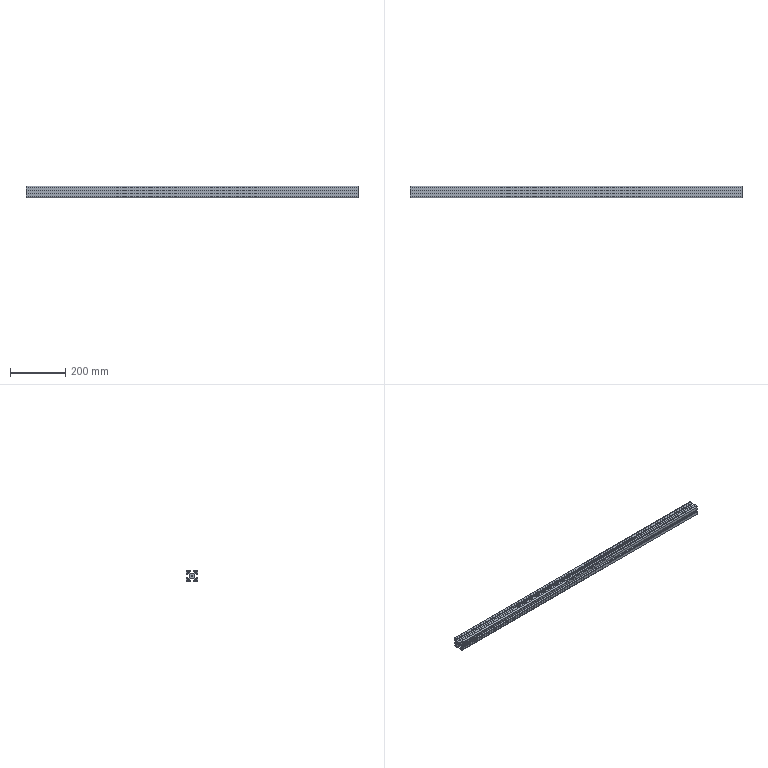Part | SolidWorks | features WeldMemberFeat 1, WeldmentFeature 1 | 1 solid | 92 faces | box 1200 x 40 x 40 mm | volume 725812 mm3 | plane 78 | cylinder 14 | commonest cylinder face diameters 6 x8 9 x4 6.8 x2